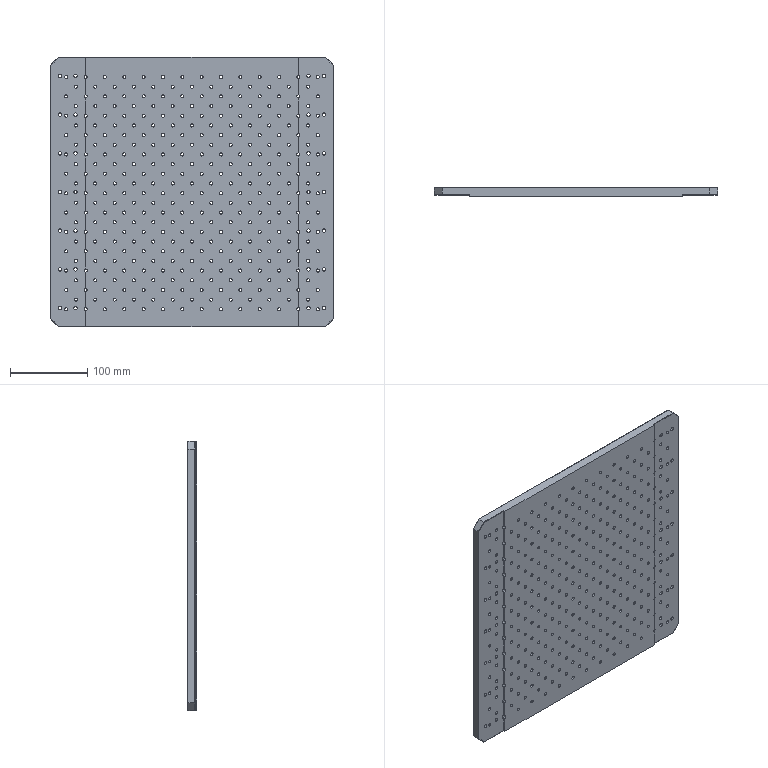Part | SolidWorks | features ICE 2, Chamfer 1, Extrusion 1, HoleWzd 1 | 1 solid | 1606 faces | box 366 x 12 x 348 mm | volume 1403273 mm3 | cylinder 788 | cone 732 | plane 86 | commonest cylinder face diameters 4 x676 4.5 x56 8 x56